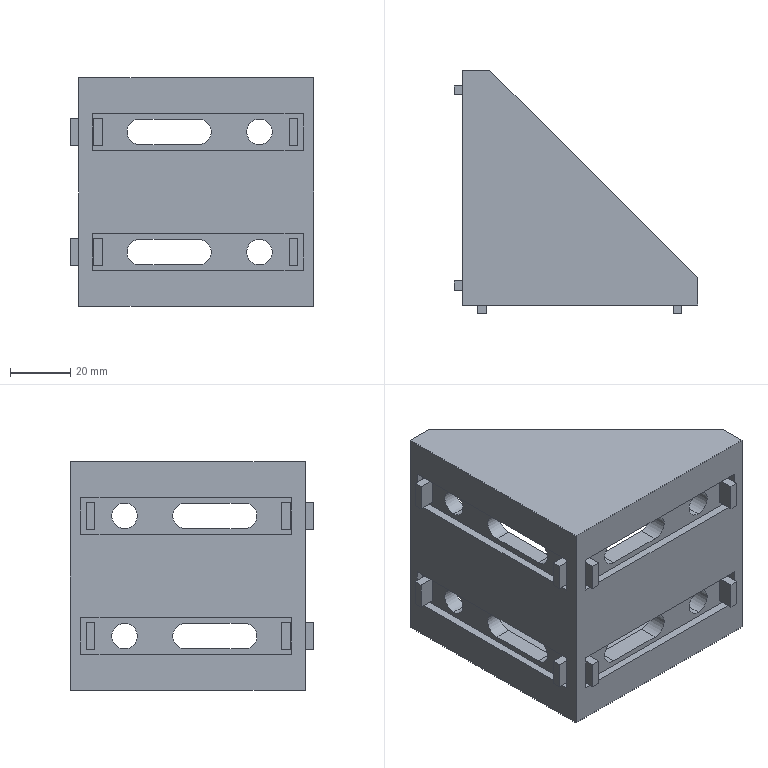Part | SolidWorks | features BaseBody 1 | 1 solid | 96 faces | box 80.8 x 80.8 x 76 mm | volume 99581 mm3 | plane 80 | cylinder 16 | commonest cylinder face diameters 8.5 x16